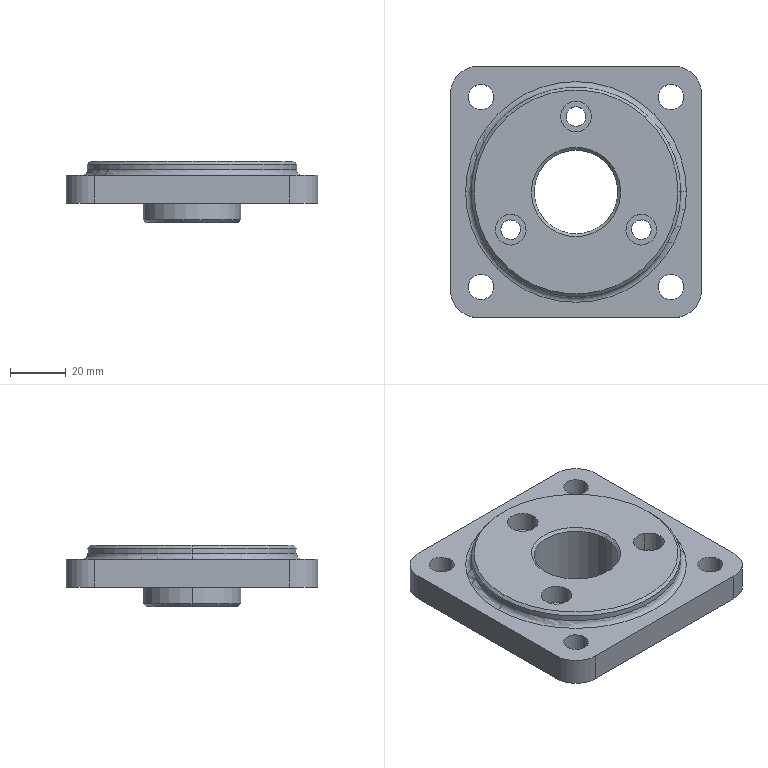Part | SolidWorks | features ICE 6, Fillet 2, Chamfer 1, CirPattern 1, Extrusion 1 | 1 solid | 49 faces | box 90 x 90 x 22 mm | volume 87928 mm3 | cylinder 30 | plane 11 | cone 6 | torus 2 | commonest cylinder face diameters 7 x6 9 x6 11 x6 20 x4 9.06 x2 30 x2
STEP:
#1=CARTESIAN_POINT('',(36.5,0.,15.));
#2=VERTEX_POINT('',#1);
#3=CARTESIAN_POINT('',(-36.5,0.,15.));
#4=VERTEX_POINT('',#3);
#5=CARTESIAN_POINT('',(0.,0.,15.));
#6=DIRECTION('',(0.,0.,1.));
#7=DIRECTION('',(1.,0.,0.));
#8=AXIS2_PLACEMENT_3D('',#5,#6,#7);
#9=CIRCLE('',#8,36.5);
#10=EDGE_CURVE('',#2,#4,#9,.T.);
#11=ORIENTED_EDGE('',*,*,#10,.F.);
#12=CARTESIAN_POINT('',(37.5,0.,14.));
#13=VERTEX_POINT('',#12);
#14=CARTESIAN_POINT('',(36.5,0.,15.));
#15=DIRECTION('',(0.7071,0.,-0.7071));
#16=VECTOR('',#15,1000.);
#17=LINE('',#14,#16);
#18=EDGE_CURVE('',#2,#13,#17,.T.);
#19=ORIENTED_EDGE('',*,*,#18,.T.);
#20=CARTESIAN_POINT('',(-37.5,0.,14.));
#21=VERTEX_POINT('',#20);
#22=CARTESIAN_POINT('',(0.,0.,14.));
#23=DIRECTION('',(0.,0.,-1.));
#24=DIRECTION('',(1.,0.,0.));
#25=AXIS2_PLACEMENT_3D('',#22,#23,#24);
#26=CIRCLE('',#25,37.5);
#27=EDGE_CURVE('',#21,#13,#26,.T.);
#28=ORIENTED_EDGE('',*,*,#27,.F.);
#29=CARTESIAN_POINT('',(-36.5,0.,15.));
#30=DIRECTION('',(-0.7071,0.,-0.7071));
#31=VECTOR('',#30,1000.);
#32=LINE('',#29,#31);
#33=EDGE_CURVE('',#4,#21,#32,.T.);
#34=ORIENTED_EDGE('',*,*,#33,.F.);
#35=EDGE_LOOP('',(#11,#19,#28,#34));
#36=FACE_OUTER_BOUND('',#35,.T.);
#37=CARTESIAN_POINT('',(0.,0.,15.));
#38=DIRECTION('',(0.,0.,-1.));
#39=DIRECTION('',(-1.,0.,0.));
#40=AXIS2_PLACEMENT_3D('',#37,#38,#39);
#41=CONICAL_SURFACE('',#40,36.5,0.7854);
#42=ADVANCED_FACE('',(#36),#41,.T.);
#43=CARTESIAN_POINT('',(-15.,0.,14.));
#44=VERTEX_POINT('',#43);
#45=CARTESIAN_POINT('',(15.,0.,14.));
#46=VERTEX_POINT('',#45);
#47=CARTESIAN_POINT('',(0.,0.,14.));
#48=DIRECTION('',(0.,0.,1.));
#49=DIRECTION('',(1.,0.,0.));
#50=AXIS2_PLACEMENT_3D('',#47,#48,#49);
#51=CIRCLE('',#50,15.);
#52=EDGE_CURVE('',#44,#46,#51,.T.);
#53=ORIENTED_EDGE('',*,*,#52,.F.);
#54=CARTESIAN_POINT('',(-16.,0.,15.));
#55=VERTEX_POINT('',#54);
#56=CARTESIAN_POINT('',(-15.,0.,14.));
#57=DIRECTION('',(-0.7071,0.,0.7071));
#58=VECTOR('',#57,1000.);
#59=LINE('',#56,#58);
#60=EDGE_CURVE('',#44,#55,#59,.T.);
#61=ORIENTED_EDGE('',*,*,#60,.T.);
#62=CARTESIAN_POINT('',(16.,0.,15.));
#63=VERTEX_POINT('',#62);
#64=CARTESIAN_POINT('',(0.,0.,15.));
#65=DIRECTION('',(0.,0.,-1.));
#66=DIRECTION('',(1.,0.,0.));
#67=AXIS2_PLACEMENT_3D('',#64,#65,#66);
#68=CIRCLE('',#67,16.);
#69=EDGE_CURVE('',#63,#55,#68,.T.);
#70=ORIENTED_EDGE('',*,*,#69,.F.);
#71=CARTESIAN_POINT('',(15.,0.,14.));
#72=DIRECTION('',(0.7071,0.,0.7071));
#73=VECTOR('',#72,1000.);
#74=LINE('',#71,#73);
#75=EDGE_CURVE('',#46,#63,#74,.T.);
#76=ORIENTED_EDGE('',*,*,#75,.F.);
#77=EDGE_LOOP('',(#53,#61,#70,#76));
#78=FACE_OUTER_BOUND('',#77,.T.);
#79=CARTESIAN_POINT('',(0.,0.,14.));
#80=DIRECTION('',(0.,0.,1.));
#81=DIRECTION('',(1.,0.,0.));
#82=AXIS2_PLACEMENT_3D('',#79,#80,#81);
#83=CONICAL_SURFACE('',#82,15.,0.7854);
#84=ADVANCED_FACE('',(#78),#83,.F.);
#85=CARTESIAN_POINT('',(-16.5,0.,-7.));
#86=VERTEX_POINT('',#85);
#87=CARTESIAN_POINT('',(16.5,0.,-7.));
#88=VERTEX_POINT('',#87);
#89=CARTESIAN_POINT('',(0.,0.,-7.));
#90=DIRECTION('',(0.,0.,-1.));
#91=DIRECTION('',(-1.,0.,0.));
#92=AXIS2_PLACEMENT_3D('',#89,#90,#91);
#93=CIRCLE('',#92,16.5);
#94=EDGE_CURVE('',#86,#88,#93,.T.);
#95=ORIENTED_EDGE('',*,*,#94,.F.);
#96=CARTESIAN_POINT('',(-17.5,0.,-6.));
#97=VERTEX_POINT('',#96);
#98=CARTESIAN_POINT('',(-16.5,0.,-7.));
#99=DIRECTION('',(-0.7071,0.,0.7071));
#100=VECTOR('',#99,1000.);
#101=LINE('',#98,#100);
#102=EDGE_CURVE('',#86,#97,#101,.T.);
#103=ORIENTED_EDGE('',*,*,#102,.T.);
#104=CARTESIAN_POINT('',(17.5,0.,-6.));
#105=VERTEX_POINT('',#104);
#106=CARTESIAN_POINT('',(0.,0.,-6.));
#107=DIRECTION('',(0.,0.,1.));
#108=DIRECTION('',(-1.,0.,0.));
#109=AXIS2_PLACEMENT_3D('',#106,#107,#108);
#110=CIRCLE('',#109,17.5);
#111=EDGE_CURVE('',#105,#97,#110,.T.);
#112=ORIENTED_EDGE('',*,*,#111,.F.);
#113=CARTESIAN_POINT('',(16.5,0.,-7.));
#114=DIRECTION('',(0.7071,0.,0.7071));
#115=VECTOR('',#114,1000.);
#116=LINE('',#113,#115);
#117=EDGE_CURVE('',#88,#105,#116,.T.);
#118=ORIENTED_EDGE('',*,*,#117,.F.);
#119=EDGE_LOOP('',(#95,#103,#112,#118));
#120=FACE_OUTER_BOUND('',#119,.T.);
#121=CARTESIAN_POINT('',(0.,0.,-7.));
#122=DIRECTION('',(0.,0.,1.));
#123=DIRECTION('',(1.,0.,0.));
#124=AXIS2_PLACEMENT_3D('',#121,#122,#123);
#125=CONICAL_SURFACE('',#124,16.5,0.7854);
#126=ADVANCED_FACE('',(#120),#125,.T.);
#127=CARTESIAN_POINT('',(-37.5,0.,12.));
#128=VERTEX_POINT('',#127);
#129=CARTESIAN_POINT('',(37.5,0.,12.));
#130=VERTEX_POINT('',#129);
#131=CARTESIAN_POINT('',(0.,0.,12.));
#132=DIRECTION('',(0.,0.,1.));
#133=DIRECTION('',(1.,0.,0.));
#134=AXIS2_PLACEMENT_3D('',#131,#132,#133);
#135=CIRCLE('',#134,37.5);
#136=EDGE_CURVE('',#128,#130,#135,.T.);
#137=ORIENTED_EDGE('',*,*,#136,.F.);
#138=CARTESIAN_POINT('',(-39.5,0.,10.));
#139=VERTEX_POINT('',#138);
#140=CARTESIAN_POINT('',(-39.5,0.,12.));
#141=DIRECTION('',(0.,1.,0.));
#142=DIRECTION('',(-1.,0.,0.));
#143=AXIS2_PLACEMENT_3D('',#140,#141,#142);
#144=CIRCLE('',#143,2.);
#145=EDGE_CURVE('',#128,#139,#144,.T.);
#146=ORIENTED_EDGE('',*,*,#145,.T.);
#147=CARTESIAN_POINT('',(39.5,0.,10.));
#148=VERTEX_POINT('',#147);
#149=CARTESIAN_POINT('',(0.,0.,10.));
#150=DIRECTION('',(0.,0.,-1.));
#151=DIRECTION('',(1.,0.,0.));
#152=AXIS2_PLACEMENT_3D('',#149,#150,#151);
#153=CIRCLE('',#152,39.5);
#154=EDGE_CURVE('',#148,#139,#153,.T.);
#155=ORIENTED_EDGE('',*,*,#154,.F.);
#156=CARTESIAN_POINT('',(39.5,0.,12.));
#157=DIRECTION('',(0.,-1.,0.));
#158=DIRECTION('',(0.,0.,-1.));
#159=AXIS2_PLACEMENT_3D('',#156,#157,#158);
#160=CIRCLE('',#159,2.);
#161=EDGE_CURVE('',#130,#148,#160,.T.);
#162=ORIENTED_EDGE('',*,*,#161,.F.);
#163=EDGE_LOOP('',(#137,#146,#155,#162));
#164=FACE_OUTER_BOUND('',#163,.T.);
#165=CARTESIAN_POINT('',(0.,0.,12.));
#166=DIRECTION('',(0.,0.,1.));
#167=DIRECTION('',(1.,0.,0.));
#168=AXIS2_PLACEMENT_3D('',#165,#166,#167);
#169=TOROIDAL_SURFACE('',#168,39.5,2.);
#170=ADVANCED_FACE('',(#164),#169,.F.);
#171=CARTESIAN_POINT('',(25.133,-10.469,0.));
#172=VERTEX_POINT('',#171);
#173=CARTESIAN_POINT('',(21.633,-16.531,0.));
#174=VERTEX_POINT('',#173);
#175=CARTESIAN_POINT('',(23.383,-13.5,0.));
#176=DIRECTION('',(0.,0.,1.));
#177=DIRECTION('',(-0.5,-0.866,0.));
#178=AXIS2_PLACEMENT_3D('',#175,#176,#177);
#179=CIRCLE('',#178,3.5);
#180=EDGE_CURVE('',#172,#174,#179,.T.);
#181=ORIENTED_EDGE('',*,*,#180,.F.);
#182=CARTESIAN_POINT('',(25.133,-10.469,8.));
#183=VERTEX_POINT('',#182);
#184=CARTESIAN_POINT('',(25.133,-10.469,-7.));
#185=DIRECTION('',(0.,0.,1.));
#186=VECTOR('',#185,1000.);
#187=LINE('',#184,#186);
#188=EDGE_CURVE('',#172,#183,#187,.T.);
#189=ORIENTED_EDGE('',*,*,#188,.T.);
#190=CARTESIAN_POINT('',(21.633,-16.531,8.));
#191=VERTEX_POINT('',#190);
#192=CARTESIAN_POINT('',(23.383,-13.5,8.));
#193=DIRECTION('',(0.,0.,1.));
#194=DIRECTION('',(-0.5,-0.866,0.));
#195=AXIS2_PLACEMENT_3D('',#192,#193,#194);
#196=CIRCLE('',#195,3.5);
#197=EDGE_CURVE('',#183,#191,#196,.T.);
#198=ORIENTED_EDGE('',*,*,#197,.T.);
#199=CARTESIAN_POINT('',(21.633,-16.531,-7.));
#200=DIRECTION('',(0.,0.,1.));
#201=VECTOR('',#200,1000.);
#202=LINE('',#199,#201);
#203=EDGE_CURVE('',#174,#191,#202,.T.);
#204=ORIENTED_EDGE('',*,*,#203,.F.);
#205=EDGE_LOOP('',(#181,#189,#198,#204));
#206=FACE_OUTER_BOUND('',#205,.T.);
#207=CARTESIAN_POINT('',(23.383,-13.5,-7.));
#208=DIRECTION('',(0.,0.,1.));
#209=DIRECTION('',(-0.5,-0.866,0.));
#210=AXIS2_PLACEMENT_3D('',#207,#208,#209);
#211=CYLINDRICAL_SURFACE('',#210,3.5);
#212=ADVANCED_FACE('',(#206),#211,.F.);
#213=CARTESIAN_POINT('',(26.133,-8.737,8.));
#214=VERTEX_POINT('',#213);
#215=CARTESIAN_POINT('',(20.633,-18.263,8.));
#216=VERTEX_POINT('',#215);
#217=CARTESIAN_POINT('',(23.383,-13.5,8.));
#218=DIRECTION('',(0.,0.,1.));
#219=DIRECTION('',(-0.5,-0.866,0.));
#220=AXIS2_PLACEMENT_3D('',#217,#218,#219);
#221=CIRCLE('',#220,5.5);
#222=EDGE_CURVE('',#214,#216,#221,.T.);
#223=ORIENTED_EDGE('',*,*,#222,.F.);
#224=CARTESIAN_POINT('',(26.133,-8.737,15.));
#225=VERTEX_POINT('',#224);
#226=CARTESIAN_POINT('',(26.133,-8.737,8.));
#227=DIRECTION('',(0.,0.,1.));
#228=VECTOR('',#227,1000.);
#229=LINE('',#226,#228);
#230=EDGE_CURVE('',#214,#225,#229,.T.);
#231=ORIENTED_EDGE('',*,*,#230,.T.);
#232=CARTESIAN_POINT('',(20.633,-18.263,15.));
#233=VERTEX_POINT('',#232);
#234=CARTESIAN_POINT('',(23.383,-13.5,15.));
#235=DIRECTION('',(0.,0.,1.));
#236=DIRECTION('',(-0.5,-0.866,0.));
#237=AXIS2_PLACEMENT_3D('',#234,#235,#236);
#238=CIRCLE('',#237,5.5);
#239=EDGE_CURVE('',#225,#233,#238,.T.);
#240=ORIENTED_EDGE('',*,*,#239,.T.);
#241=CARTESIAN_POINT('',(20.633,-18.263,8.));
#242=DIRECTION('',(0.,0.,1.));
#243=VECTOR('',#242,1000.);
#244=LINE('',#241,#243);
#245=EDGE_CURVE('',#216,#233,#244,.T.);
#246=ORIENTED_EDGE('',*,*,#245,.F.);
#247=EDGE_LOOP('',(#223,#231,#240,#246));
#248=FACE_OUTER_BOUND('',#247,.T.);
#249=CARTESIAN_POINT('',(23.383,-13.5,8.));
#250=DIRECTION('',(0.,0.,1.));
#251=DIRECTION('',(-0.5,-0.866,0.));
#252=AXIS2_PLACEMENT_3D('',#249,#250,#251);
#253=CYLINDRICAL_SURFACE('',#252,5.5);
#254=ADVANCED_FACE('',(#248),#253,.F.);
#255=CARTESIAN_POINT('',(-21.633,-16.531,0.));
#256=VERTEX_POINT('',#255);
#257=CARTESIAN_POINT('',(-25.133,-10.469,0.));
#258=VERTEX_POINT('',#257);
#259=CARTESIAN_POINT('',(-23.383,-13.5,0.));
#260=DIRECTION('',(0.,0.,1.));
#261=DIRECTION('',(-0.5,0.866,0.));
#262=AXIS2_PLACEMENT_3D('',#259,#260,#261);
#263=CIRCLE('',#262,3.5);
#264=EDGE_CURVE('',#256,#258,#263,.T.);
#265=ORIENTED_EDGE('',*,*,#264,.F.);
#266=CARTESIAN_POINT('',(-21.633,-16.531,8.));
#267=VERTEX_POINT('',#266);
#268=CARTESIAN_POINT('',(-21.633,-16.531,-7.));
#269=DIRECTION('',(0.,0.,1.));
#270=VECTOR('',#269,1000.);
#271=LINE('',#268,#270);
#272=EDGE_CURVE('',#256,#267,#271,.T.);
#273=ORIENTED_EDGE('',*,*,#272,.T.);
#274=CARTESIAN_POINT('',(-25.133,-10.469,8.));
#275=VERTEX_POINT('',#274);
#276=CARTESIAN_POINT('',(-23.383,-13.5,8.));
#277=DIRECTION('',(0.,0.,1.));
#278=DIRECTION('',(-0.5,0.866,0.));
#279=AXIS2_PLACEMENT_3D('',#276,#277,#278);
#280=CIRCLE('',#279,3.5);
#281=EDGE_CURVE('',#267,#275,#280,.T.);
#282=ORIENTED_EDGE('',*,*,#281,.T.);
#283=CARTESIAN_POINT('',(-25.133,-10.469,-7.));
#284=DIRECTION('',(0.,0.,1.));
#285=VECTOR('',#284,1000.);
#286=LINE('',#283,#285);
#287=EDGE_CURVE('',#258,#275,#286,.T.);
#288=ORIENTED_EDGE('',*,*,#287,.F.);
#289=EDGE_LOOP('',(#265,#273,#282,#288));
#290=FACE_OUTER_BOUND('',#289,.T.);
#291=CARTESIAN_POINT('',(-23.383,-13.5,-7.));
#292=DIRECTION('',(0.,0.,1.));
#293=DIRECTION('',(-0.5,0.866,0.));
#294=AXIS2_PLACEMENT_3D('',#291,#292,#293);
#295=CYLINDRICAL_SURFACE('',#294,3.5);
#296=ADVANCED_FACE('',(#290),#295,.F.);
#297=CARTESIAN_POINT('',(-20.633,-18.263,8.));
#298=VERTEX_POINT('',#297);
#299=CARTESIAN_POINT('',(-26.133,-8.737,8.));
#300=VERTEX_POINT('',#299);
#301=CARTESIAN_POINT('',(-23.383,-13.5,8.));
#302=DIRECTION('',(0.,0.,1.));
#303=DIRECTION('',(-0.5,0.866,0.));
#304=AXIS2_PLACEMENT_3D('',#301,#302,#303);
#305=CIRCLE('',#304,5.5);
#306=EDGE_CURVE('',#298,#300,#305,.T.);
#307=ORIENTED_EDGE('',*,*,#306,.F.);
#308=CARTESIAN_POINT('',(-20.633,-18.263,15.));
#309=VERTEX_POINT('',#308);
#310=CARTESIAN_POINT('',(-20.633,-18.263,8.));
#311=DIRECTION('',(0.,0.,1.));
#312=VECTOR('',#311,1000.);
#313=LINE('',#310,#312);
#314=EDGE_CURVE('',#298,#309,#313,.T.);
#315=ORIENTED_EDGE('',*,*,#314,.T.);
#316=CARTESIAN_POINT('',(-26.133,-8.737,15.));
#317=VERTEX_POINT('',#316);
#318=CARTESIAN_POINT('',(-23.383,-13.5,15.));
#319=DIRECTION('',(0.,0.,1.));
#320=DIRECTION('',(-0.5,0.866,0.));
#321=AXIS2_PLACEMENT_3D('',#318,#319,#320);
#322=CIRCLE('',#321,5.5);
#323=EDGE_CURVE('',#309,#317,#322,.T.);
#324=ORIENTED_EDGE('',*,*,#323,.T.);
#325=CARTESIAN_POINT('',(-26.133,-8.737,8.));
#326=DIRECTION('',(0.,0.,1.));
#327=VECTOR('',#326,1000.);
#328=LINE('',#325,#327);
#329=EDGE_CURVE('',#300,#317,#328,.T.);
#330=ORIENTED_EDGE('',*,*,#329,.F.);
#331=EDGE_LOOP('',(#307,#315,#324,#330));
#332=FACE_OUTER_BOUND('',#331,.T.);
#333=CARTESIAN_POINT('',(-23.383,-13.5,8.));
#334=DIRECTION('',(0.,0.,1.));
#335=DIRECTION('',(-0.5,0.866,0.));
#336=AXIS2_PLACEMENT_3D('',#333,#334,#335);
#337=CYLINDRICAL_SURFACE('',#336,5.5);
#338=ADVANCED_FACE('',(#332),#337,.F.);
#339=CARTESIAN_POINT('',(-3.5,27.,0.));
#340=VERTEX_POINT('',#339);
#341=CARTESIAN_POINT('',(3.5,27.,0.));
#342=VERTEX_POINT('',#341);
#343=CARTESIAN_POINT('',(0.,27.,0.));
#344=DIRECTION('',(0.,0.,1.));
#345=DIRECTION('',(1.,0.,0.));
#346=AXIS2_PLACEMENT_3D('',#343,#344,#345);
#347=CIRCLE('',#346,3.5);
#348=EDGE_CURVE('',#340,#342,#347,.T.);
#349=ORIENTED_EDGE('',*,*,#348,.F.);
#350=CARTESIAN_POINT('',(-3.5,27.,8.));
#351=VERTEX_POINT('',#350);
#352=CARTESIAN_POINT('',(-3.5,27.,-7.));
#353=DIRECTION('',(0.,0.,1.));
#354=VECTOR('',#353,1000.);
#355=LINE('',#352,#354);
#356=EDGE_CURVE('',#340,#351,#355,.T.);
#357=ORIENTED_EDGE('',*,*,#356,.T.);
#358=CARTESIAN_POINT('',(3.5,27.,8.));
#359=VERTEX_POINT('',#358);
#360=CARTESIAN_POINT('',(0.,27.,8.));
#361=DIRECTION('',(0.,0.,1.));
#362=DIRECTION('',(1.,0.,0.));
#363=AXIS2_PLACEMENT_3D('',#360,#361,#362);
#364=CIRCLE('',#363,3.5);
#365=EDGE_CURVE('',#351,#359,#364,.T.);
#366=ORIENTED_EDGE('',*,*,#365,.T.);
#367=CARTESIAN_POINT('',(3.5,27.,-7.));
#368=DIRECTION('',(0.,0.,1.));
#369=VECTOR('',#368,1000.);
#370=LINE('',#367,#369);
#371=EDGE_CURVE('',#342,#359,#370,.T.);
#372=ORIENTED_EDGE('',*,*,#371,.F.);
#373=EDGE_LOOP('',(#349,#357,#366,#372));
#374=FACE_OUTER_BOUND('',#373,.T.);
#375=CARTESIAN_POINT('',(0.,27.,-7.));
#376=DIRECTION('',(0.,0.,1.));
#377=DIRECTION('',(1.,0.,0.));
#378=AXIS2_PLACEMENT_3D('',#375,#376,#377);
#379=CYLINDRICAL_SURFACE('',#378,3.5);
#380=ADVANCED_FACE('',(#374),#379,.F.);
#381=CARTESIAN_POINT('',(-5.5,27.,8.));
#382=VERTEX_POINT('',#381);
#383=CARTESIAN_POINT('',(5.5,27.,8.));
#384=VERTEX_POINT('',#383);
#385=CARTESIAN_POINT('',(0.,27.,8.));
#386=DIRECTION('',(0.,0.,1.));
#387=DIRECTION('',(1.,0.,0.));
#388=AXIS2_PLACEMENT_3D('',#385,#386,#387);
#389=CIRCLE('',#388,5.5);
#390=EDGE_CURVE('',#382,#384,#389,.T.);
#391=ORIENTED_EDGE('',*,*,#390,.F.);
#392=CARTESIAN_POINT('',(-5.5,27.,15.));
#393=VERTEX_POINT('',#392);
#394=CARTESIAN_POINT('',(-5.5,27.,8.));
#395=DIRECTION('',(0.,0.,1.));
#396=VECTOR('',#395,1000.);
#397=LINE('',#394,#396);
#398=EDGE_CURVE('',#382,#393,#397,.T.);
#399=ORIENTED_EDGE('',*,*,#398,.T.);
#400=CARTESIAN_POINT('',(5.5,27.,15.));
#401=VERTEX_POINT('',#400);
#402=CARTESIAN_POINT('',(0.,27.,15.));
#403=DIRECTION('',(0.,0.,1.));
#404=DIRECTION('',(1.,0.,0.));
#405=AXIS2_PLACEMENT_3D('',#402,#403,#404);
#406=CIRCLE('',#405,5.5);
#407=EDGE_CURVE('',#393,#401,#406,.T.);
#408=ORIENTED_EDGE('',*,*,#407,.T.);
#409=CARTESIAN_POINT('',(5.5,27.,8.));
#410=DIRECTION('',(0.,0.,1.));
#411=VECTOR('',#410,1000.);
#412=LINE('',#409,#411);
#413=EDGE_CURVE('',#384,#401,#412,.T.);
#414=ORIENTED_EDGE('',*,*,#413,.F.);
#415=EDGE_LOOP('',(#391,#399,#408,#414));
#416=FACE_OUTER_BOUND('',#415,.T.);
#417=CARTESIAN_POINT('',(0.,27.,8.));
#418=DIRECTION('',(0.,0.,1.));
#419=DIRECTION('',(1.,0.,0.));
#420=AXIS2_PLACEMENT_3D('',#417,#418,#419);
#421=CYLINDRICAL_SURFACE('',#420,5.5);
#422=ADVANCED_FACE('',(#416),#421,.F.);
#423=CARTESIAN_POINT('',(-15.,0.,-7.));
#424=VERTEX_POINT('',#423);
#425=CARTESIAN_POINT('',(15.,0.,-7.));
#426=VERTEX_POINT('',#425);
#427=CARTESIAN_POINT('',(0.,0.,-7.));
#428=DIRECTION('',(0.,0.,1.));
#429=DIRECTION('',(1.,0.,0.));
#430=AXIS2_PLACEMENT_3D('',#427,#428,#429);
#431=CIRCLE('',#430,15.);
#432=EDGE_CURVE('',#424,#426,#431,.T.);
#433=ORIENTED_EDGE('',*,*,#432,.F.);
#434=CARTESIAN_POINT('',(-15.,0.,-7.));
#435=DIRECTION('',(0.,0.,1.));
#436=VECTOR('',#435,1000.);
#437=LINE('',#434,#436);
#438=EDGE_CURVE('',#424,#44,#437,.T.);
#439=ORIENTED_EDGE('',*,*,#438,.T.);
#440=ORIENTED_EDGE('',*,*,#52,.T.);
#441=CARTESIAN_POINT('',(15.,0.,-7.));
#442=DIRECTION('',(0.,0.,1.));
#443=VECTOR('',#442,1000.);
#444=LINE('',#441,#443);
#445=EDGE_CURVE('',#426,#46,#444,.T.);
#446=ORIENTED_EDGE('',*,*,#445,.F.);
#447=EDGE_LOOP('',(#433,#439,#440,#446));
#448=FACE_OUTER_BOUND('',#447,.T.);
#449=CARTESIAN_POINT('',(0.,0.,-7.));
#450=DIRECTION('',(0.,0.,1.));
#451=DIRECTION('',(1.,0.,0.));
#452=AXIS2_PLACEMENT_3D('',#449,#450,#451);
#453=CYLINDRICAL_SURFACE('',#452,15.);
#454=ADVANCED_FACE('',(#448),#453,.F.);
#455=ORIENTED_EDGE('',*,*,#111,.T.);
#456=CARTESIAN_POINT('',(-17.5,0.,0.));
#457=VERTEX_POINT('',#456);
#458=CARTESIAN_POINT('',(-17.5,0.,-7.));
#459=DIRECTION('',(0.,0.,1.));
#460=VECTOR('',#459,1000.);
#461=LINE('',#458,#460);
#462=EDGE_CURVE('',#97,#457,#461,.T.);
#463=ORIENTED_EDGE('',*,*,#462,.T.);
#464=CARTESIAN_POINT('',(17.5,0.,0.));
#465=VERTEX_POINT('',#464);
#466=CARTESIAN_POINT('',(0.,0.,0.));
#467=DIRECTION('',(0.,0.,-1.));
#468=DIRECTION('',(1.,0.,0.));
#469=AXIS2_PLACEMENT_3D('',#466,#467,#468);
#470=CIRCLE('',#469,17.5);
#471=EDGE_CURVE('',#457,#465,#470,.T.);
#472=ORIENTED_EDGE('',*,*,#471,.T.);
#473=CARTESIAN_POINT('',(17.5,0.,-7.));
#474=DIRECTION('',(0.,0.,1.));
#475=VECTOR('',#474,1000.);
#476=LINE('',#473,#475);
#477=EDGE_CURVE('',#105,#465,#476,.T.);
#478=ORIENTED_EDGE('',*,*,#477,.F.);
#479=EDGE_LOOP('',(#455,#463,#472,#478));
#480=FACE_OUTER_BOUND('',#479,.T.);
#481=CARTESIAN_POINT('',(0.,0.,-7.));
#482=DIRECTION('',(0.,0.,1.));
#483=DIRECTION('',(1.,0.,0.));
#484=AXIS2_PLACEMENT_3D('',#481,#482,#483);
#485=CYLINDRICAL_SURFACE('',#484,17.5);
#486=ADVANCED_FACE('',(#480),#485,.T.);
#487=ORIENTED_EDGE('',*,*,#27,.T.);
#488=CARTESIAN_POINT('',(37.5,0.,15.));
#489=DIRECTION('',(0.,0.,-1.));
#490=VECTOR('',#489,1000.);
#491=LINE('',#488,#490);
#492=EDGE_CURVE('',#13,#130,#491,.T.);
#493=ORIENTED_EDGE('',*,*,#492,.T.);
#494=CARTESIAN_POINT('',(0.,0.,12.));
#495=DIRECTION('',(0.,0.,1.));
#496=DIRECTION('',(1.,0.,0.));
#497=AXIS2_PLACEMENT_3D('',#494,#495,#496);
#498=CIRCLE('',#497,37.5);
#499=EDGE_CURVE('',#130,#128,#498,.T.);
#500=ORIENTED_EDGE('',*,*,#499,.T.);
#501=CARTESIAN_POINT('',(-37.5,0.,15.));
#502=DIRECTION('',(0.,0.,-1.));
#503=VECTOR('',#502,1000.);
#504=LINE('',#501,#503);
#505=EDGE_CURVE('',#21,#128,#504,.T.);
#506=ORIENTED_EDGE('',*,*,#505,.F.);
#507=EDGE_LOOP('',(#487,#493,#500,#506));
#508=FACE_OUTER_BOUND('',#507,.T.);
#509=CARTESIAN_POINT('',(0.,0.,15.));
#510=DIRECTION('',(0.,0.,-1.));
#511=DIRECTION('',(-1.,0.,0.));
#512=AXIS2_PLACEMENT_3D('',#509,#510,#511);
#513=CYLINDRICAL_SURFACE('',#512,37.5);
#514=ADVANCED_FACE('',(#508),#513,.T.);
#515=CARTESIAN_POINT('',(29.5,34.,0.));
#516=VERTEX_POINT('',#515);
#517=CARTESIAN_POINT('',(38.5,34.,0.));
#518=VERTEX_POINT('',#517);
#519=CARTESIAN_POINT('',(34.,34.,0.));
#520=DIRECTION('',(0.,0.,1.));
#521=DIRECTION('',(1.,0.,0.));
#522=AXIS2_PLACEMENT_3D('',#519,#520,#521);
#523=CIRCLE('',#522,4.5);
#524=EDGE_CURVE('',#516,#518,#523,.T.);
#525=ORIENTED_EDGE('',*,*,#524,.F.);
#526=CARTESIAN_POINT('',(29.5,34.,10.));
#527=VERTEX_POINT('',#526);
#528=CARTESIAN_POINT('',(29.5,34.,0.));
#529=DIRECTION('',(0.,0.,1.));
#530=VECTOR('',#529,1000.);
#531=LINE('',#528,#530);
#532=EDGE_CURVE('',#516,#527,#531,.T.);
#533=ORIENTED_EDGE('',*,*,#532,.T.);
#534=CARTESIAN_POINT('',(38.5,34.,10.));
#535=VERTEX_POINT('',#534);
#536=CARTESIAN_POINT('',(34.,34.,10.));
#537=DIRECTION('',(0.,0.,1.));
#538=DIRECTION('',(1.,0.,0.));
#539=AXIS2_PLACEMENT_3D('',#536,#537,#538);
#540=CIRCLE('',#539,4.5);
#541=EDGE_CURVE('',#527,#535,#540,.T.);
#542=ORIENTED_EDGE('',*,*,#541,.T.);
#543=CARTESIAN_POINT('',(38.5,34.,0.));
#544=DIRECTION('',(0.,0.,1.));
#545=VECTOR('',#544,1000.);
#546=LINE('',#543,#545);
#547=EDGE_CURVE('',#518,#535,#546,.T.);
#548=ORIENTED_EDGE('',*,*,#547,.F.);
#549=EDGE_LOOP('',(#525,#533,#542,#548));
#550=FACE_OUTER_BOUND('',#549,.T.);
#551=CARTESIAN_POINT('',(34.,34.,0.));
#552=DIRECTION('',(0.,0.,1.));
#553=DIRECTION('',(1.,0.,0.));
#554=AXIS2_PLACEMENT_3D('',#551,#552,#553);
#555=CYLINDRICAL_SURFACE('',#554,4.5);
#556=ADVANCED_FACE('',(#550),#555,.F.);
#557=CARTESIAN_POINT('',(-38.5,-34.,0.));
#558=VERTEX_POINT('',#557);
#559=CARTESIAN_POINT('',(-29.5,-34.,0.));
#560=VERTEX_POINT('',#559);
#561=CARTESIAN_POINT('',(-34.,-34.,0.));
#562=DIRECTION('',(0.,0.,1.));
#563=DIRECTION('',(1.,0.,0.));
#564=AXIS2_PLACEMENT_3D('',#561,#562,#563);
#565=CIRCLE('',#564,4.5);
#566=EDGE_CURVE('',#558,#560,#565,.T.);
#567=ORIENTED_EDGE('',*,*,#566,.F.);
#568=CARTESIAN_POINT('',(-38.5,-34.,10.));
#569=VERTEX_POINT('',#568);
#570=CARTESIAN_POINT('',(-38.5,-34.,0.));
#571=DIRECTION('',(0.,0.,1.));
#572=VECTOR('',#571,1000.);
#573=LINE('',#570,#572);
#574=EDGE_CURVE('',#558,#569,#573,.T.);
#575=ORIENTED_EDGE('',*,*,#574,.T.);
#576=CARTESIAN_POINT('',(-29.5,-34.,10.));
#577=VERTEX_POINT('',#576);
#578=CARTESIAN_POINT('',(-34.,-34.,10.));
#579=DIRECTION('',(0.,0.,1.));
#580=DIRECTION('',(1.,0.,0.));
#581=AXIS2_PLACEMENT_3D('',#578,#579,#580);
#582=CIRCLE('',#581,4.5);
#583=EDGE_CURVE('',#569,#577,#582,.T.);
#584=ORIENTED_EDGE('',*,*,#583,.T.);
#585=CARTESIAN_POINT('',(-29.5,-34.,0.));
#586=DIRECTION('',(0.,0.,1.));
#587=VECTOR('',#586,1000.);
#588=LINE('',#585,#587);
#589=EDGE_CURVE('',#560,#577,#588,.T.);
#590=ORIENTED_EDGE('',*,*,#589,.F.);
#591=EDGE_LOOP('',(#567,#575,#584,#590));
#592=FACE_OUTER_BOUND('',#591,.T.);
#593=CARTESIAN_POINT('',(-34.,-34.,0.));
#594=DIRECTION('',(0.,0.,1.));
#595=DIRECTION('',(1.,0.,0.));
#596=AXIS2_PLACEMENT_3D('',#593,#594,#595);
#597=CYLINDRICAL_SURFACE('',#596,4.5);
#598=ADVANCED_FACE('',(#592),#597,.F.);
#599=CARTESIAN_POINT('',(29.47,-34.,0.));
#600=VERTEX_POINT('',#599);
#601=CARTESIAN_POINT('',(38.53,-34.,0.));
#602=VERTEX_POINT('',#601);
#603=CARTESIAN_POINT('',(34.,-34.,0.));
#604=DIRECTION('',(0.,0.,1.));
#605=DIRECTION('',(1.,0.,0.));
#606=AXIS2_PLACEMENT_3D('',#603,#604,#605);
#607=CIRCLE('',#606,4.53);
#608=EDGE_CURVE('',#600,#602,#607,.T.);
#609=ORIENTED_EDGE('',*,*,#608,.F.);
#610=CARTESIAN_POINT('',(29.47,-34.,10.));
#611=VERTEX_POINT('',#610);
#612=CARTESIAN_POINT('',(29.47,-34.,0.));
#613=DIRECTION('',(0.,0.,1.));
#614=VECTOR('',#613,1000.);
#615=LINE('',#612,#614);
#616=EDGE_CURVE('',#600,#611,#615,.T.);
#617=ORIENTED_EDGE('',*,*,#616,.T.);
#618=CARTESIAN_POINT('',(38.53,-34.,10.));
#619=VERTEX_POINT('',#618);
#620=CARTESIAN_POINT('',(34.,-34.,10.));
#621=DIRECTION('',(0.,0.,1.));
#622=DIRECTION('',(1.,0.,0.));
#623=AXIS2_PLACEMENT_3D('',#620,#621,#622);
#624=CIRCLE('',#623,4.53);
#625=EDGE_CURVE('',#611,#619,#624,.T.);
#626=ORIENTED_EDGE('',*,*,#625,.T.);
#627=CARTESIAN_POINT('',(38.53,-34.,0.));
#628=DIRECTION('',(0.,0.,1.));
#629=VECTOR('',#628,1000.);
#630=LINE('',#627,#629);
#631=EDGE_CURVE('',#602,#619,#630,.T.);
#632=ORIENTED_EDGE('',*,*,#631,.F.);
#633=EDGE_LOOP('',(#609,#617,#626,#632));
#634=FACE_OUTER_BOUND('',#633,.T.);
#635=CARTESIAN_POINT('',(34.,-34.,0.));
#636=DIRECTION('',(0.,0.,1.));
#637=DIRECTION('',(1.,0.,0.));
#638=AXIS2_PLACEMENT_3D('',#635,#636,#637);
#639=CYLINDRICAL_SURFACE('',#638,4.53);
#640=ADVANCED_FACE('',(#634),#639,.F.);
#641=CARTESIAN_POINT('',(-38.5,34.,0.));
#642=VERTEX_POINT('',#641);
#643=CARTESIAN_POINT('',(-29.5,34.,0.));
#644=VERTEX_POINT('',#643);
#645=CARTESIAN_POINT('',(-34.,34.,0.));
#646=DIRECTION('',(0.,0.,1.));
#647=DIRECTION('',(1.,0.,0.));
#648=AXIS2_PLACEMENT_3D('',#645,#646,#647);
#649=CIRCLE('',#648,4.5);
#650=EDGE_CURVE('',#642,#644,#649,.T.);
#651=ORIENTED_EDGE('',*,*,#650,.F.);
#652=CARTESIAN_POINT('',(-38.5,34.,10.));
#653=VERTEX_POINT('',#652);
#654=CARTESIAN_POINT('',(-38.5,34.,0.));
#655=DIRECTION('',(0.,0.,1.));
#656=VECTOR('',#655,1000.);
#657=LINE('',#654,#656);
#658=EDGE_CURVE('',#642,#653,#657,.T.);
#659=ORIENTED_EDGE('',*,*,#658,.T.);
#660=CARTESIAN_POINT('',(-29.5,34.,10.));
#661=VERTEX_POINT('',#660);
#662=CARTESIAN_POINT('',(-34.,34.,10.));
#663=DIRECTION('',(0.,0.,1.));
#664=DIRECTION('',(1.,0.,0.));
#665=AXIS2_PLACEMENT_3D('',#662,#663,#664);
#666=CIRCLE('',#665,4.5);
#667=EDGE_CURVE('',#653,#661,#666,.T.);
#668=ORIENTED_EDGE('',*,*,#667,.T.);
#669=CARTESIAN_POINT('',(-29.5,34.,0.));
#670=DIRECTION('',(0.,0.,1.));
#671=VECTOR('',#670,1000.);
#672=LINE('',#669,#671);
#673=EDGE_CURVE('',#644,#661,#672,.T.);
#674=ORIENTED_EDGE('',*,*,#673,.F.);
#675=EDGE_LOOP('',(#651,#659,#668,#674));
#676=FACE_OUTER_BOUND('',#675,.T.);
#677=CARTESIAN_POINT('',(-34.,34.,0.));
#678=DIRECTION('',(0.,0.,1.));
#679=DIRECTION('',(1.,0.,0.));
#680=AXIS2_PLACEMENT_3D('',#677,#678,#679);
#681=CYLINDRICAL_SURFACE('',#680,4.5);
#682=ADVANCED_FACE('',(#676),#681,.F.);
#683=CARTESIAN_POINT('',(45.,-35.,10.));
#684=VERTEX_POINT('',#683);
#685=CARTESIAN_POINT('',(45.,35.,10.));
#686=VERTEX_POINT('',#685);
#687=CARTESIAN_POINT('',(45.,45.,10.));
#688=DIRECTION('',(0.,1.,0.));
#689=VECTOR('',#688,1000.);
#690=LINE('',#687,#689);
#691=EDGE_CURVE('',#684,#686,#690,.T.);
#692=ORIENTED_EDGE('',*,*,#691,.F.);
#693=CARTESIAN_POINT('',(45.,-35.,0.));
#694=VERTEX_POINT('',#693);
#695=CARTESIAN_POINT('',(45.,-35.,10.));
#696=DIRECTION('',(0.,0.,-1.));
#697=VECTOR('',#696,1000.);
#698=LINE('',#695,#697);
#699=EDGE_CURVE('',#684,#694,#698,.T.);
#700=ORIENTED_EDGE('',*,*,#699,.T.);
#701=CARTESIAN_POINT('',(45.,35.,0.));
#702=VERTEX_POINT('',#701);
#703=CARTESIAN_POINT('',(45.,45.,0.));
#704=DIRECTION('',(0.,1.,0.));
#705=VECTOR('',#704,1000.);
#706=LINE('',#703,#705);
#707=EDGE_CURVE('',#694,#702,#706,.T.);
#708=ORIENTED_EDGE('',*,*,#707,.T.);
#709=CARTESIAN_POINT('',(45.,35.,10.));
#710=DIRECTION('',(0.,0.,1.));
#711=VECTOR('',#710,1000.);
#712=LINE('',#709,#711);
#713=EDGE_CURVE('',#702,#686,#712,.T.);
#714=ORIENTED_EDGE('',*,*,#713,.T.);
#715=EDGE_LOOP('',(#692,#700,#708,#714));
#716=FACE_OUTER_BOUND('',#715,.T.);
#717=CARTESIAN_POINT('',(45.,45.,10.));
#718=DIRECTION('',(-1.,0.,0.));
#719=DIRECTION('',(0.,-1.,0.));
#720=AXIS2_PLACEMENT_3D('',#717,#718,#719);
#721=PLANE('',#720);
#722=ADVANCED_FACE('',(#716),#721,.F.);
#723=CARTESIAN_POINT('',(35.,45.,10.));
#724=VERTEX_POINT('',#723);
#725=CARTESIAN_POINT('',(-35.,45.,10.));
#726=VERTEX_POINT('',#725);
#727=CARTESIAN_POINT('',(-45.,45.,10.));
#728=DIRECTION('',(-1.,0.,0.));
#729=VECTOR('',#728,1000.);
#730=LINE('',#727,#729);
#731=EDGE_CURVE('',#724,#726,#730,.T.);
#732=ORIENTED_EDGE('',*,*,#731,.F.);
#733=CARTESIAN_POINT('',(35.,45.,0.));
#734=VERTEX_POINT('',#733);
#735=CARTESIAN_POINT('',(35.,45.,10.));
#736=DIRECTION('',(0.,0.,-1.));
#737=VECTOR('',#736,1000.);
#738=LINE('',#735,#737);
#739=EDGE_CURVE('',#724,#734,#738,.T.);
#740=ORIENTED_EDGE('',*,*,#739,.T.);
#741=CARTESIAN_POINT('',(-35.,45.,0.));
#742=VERTEX_POINT('',#741);
#743=CARTESIAN_POINT('',(-45.,45.,0.));
#744=DIRECTION('',(-1.,0.,0.));
#745=VECTOR('',#744,1000.);
#746=LINE('',#743,#745);
#747=EDGE_CURVE('',#734,#742,#746,.T.);
#748=ORIENTED_EDGE('',*,*,#747,.T.);
#749=CARTESIAN_POINT('',(-35.,45.,10.));
#750=DIRECTION('',(0.,0.,1.));
#751=VECTOR('',#750,1000.);
#752=LINE('',#749,#751);
#753=EDGE_CURVE('',#742,#726,#752,.T.);
#754=ORIENTED_EDGE('',*,*,#753,.T.);
#755=EDGE_LOOP('',(#732,#740,#748,#754));
#756=FACE_OUTER_BOUND('',#755,.T.);
#757=CARTESIAN_POINT('',(-45.,45.,10.));
#758=DIRECTION('',(0.,-1.,0.));
#759=DIRECTION('',(0.,0.,-1.));
#760=AXIS2_PLACEMENT_3D('',#757,#758,#759);
#761=PLANE('',#760);
#762=ADVANCED_FACE('',(#756),#761,.F.);
#763=CARTESIAN_POINT('',(-45.,35.,0.));
#764=VERTEX_POINT('',#763);
#765=CARTESIAN_POINT('',(-45.,-35.,0.));
#766=VERTEX_POINT('',#765);
#767=CARTESIAN_POINT('',(-45.,45.,0.));
#768=DIRECTION('',(0.,-1.,0.));
#769=VECTOR('',#768,1000.);
#770=LINE('',#767,#769);
#771=EDGE_CURVE('',#764,#766,#770,.T.);
#772=ORIENTED_EDGE('',*,*,#771,.T.);
#773=CARTESIAN_POINT('',(-45.,-35.,10.));
#774=VERTEX_POINT('',#773);
#775=CARTESIAN_POINT('',(-45.,-35.,10.));
#776=DIRECTION('',(0.,0.,1.));
#777=VECTOR('',#776,1000.);
#778=LINE('',#775,#777);
#779=EDGE_CURVE('',#766,#774,#778,.T.);
#780=ORIENTED_EDGE('',*,*,#779,.T.);
#781=CARTESIAN_POINT('',(-45.,35.,10.));
#782=VERTEX_POINT('',#781);
#783=CARTESIAN_POINT('',(-45.,45.,10.));
#784=DIRECTION('',(0.,-1.,0.));
#785=VECTOR('',#784,1000.);
#786=LINE('',#783,#785);
#787=EDGE_CURVE('',#782,#774,#786,.T.);
#788=ORIENTED_EDGE('',*,*,#787,.F.);
#789=CARTESIAN_POINT('',(-45.,35.,10.));
#790=DIRECTION('',(0.,0.,-1.));
#791=VECTOR('',#790,1000.);
#792=LINE('',#789,#791);
#793=EDGE_CURVE('',#782,#764,#792,.T.);
#794=ORIENTED_EDGE('',*,*,#793,.T.);
#795=EDGE_LOOP('',(#772,#780,#788,#794));
#796=FACE_OUTER_BOUND('',#795,.T.);
#797=CARTESIAN_POINT('',(-45.,45.,10.));
#798=DIRECTION('',(1.,0.,0.));
#799=DIRECTION('',(0.,1.,0.));
#800=AXIS2_PLACEMENT_3D('',#797,#798,#799);
#801=PLANE('',#800);
#802=ADVANCED_FACE('',(#796),#801,.F.);
#803=CARTESIAN_POINT('',(-35.,-45.,10.));
#804=VERTEX_POINT('',#803);
#805=CARTESIAN_POINT('',(35.,-45.,10.));
#806=VERTEX_POINT('',#805);
#807=CARTESIAN_POINT('',(-45.,-45.,10.));
#808=DIRECTION('',(1.,0.,0.));
#809=VECTOR('',#808,1000.);
#810=LINE('',#807,#809);
#811=EDGE_CURVE('',#804,#806,#810,.T.);
#812=ORIENTED_EDGE('',*,*,#811,.F.);
#813=CARTESIAN_POINT('',(-35.,-45.,0.));
#814=VERTEX_POINT('',#813);
#815=CARTESIAN_POINT('',(-35.,-45.,10.));
#816=DIRECTION('',(0.,0.,-1.));
#817=VECTOR('',#816,1000.);
#818=LINE('',#815,#817);
#819=EDGE_CURVE('',#804,#814,#818,.T.);
#820=ORIENTED_EDGE('',*,*,#819,.T.);
#821=CARTESIAN_POINT('',(35.,-45.,0.));
#822=VERTEX_POINT('',#821);
#823=CARTESIAN_POINT('',(-45.,-45.,0.));
#824=DIRECTION('',(1.,0.,0.));
#825=VECTOR('',#824,1000.);
#826=LINE('',#823,#825);
#827=EDGE_CURVE('',#814,#822,#826,.T.);
#828=ORIENTED_EDGE('',*,*,#827,.T.);
#829=CARTESIAN_POINT('',(35.,-45.,10.));
#830=DIRECTION('',(0.,0.,1.));
#831=VECTOR('',#830,1000.);
#832=LINE('',#829,#831);
#833=EDGE_CURVE('',#822,#806,#832,.T.);
#834=ORIENTED_EDGE('',*,*,#833,.T.);
#835=EDGE_LOOP('',(#812,#820,#828,#834));
#836=FACE_OUTER_BOUND('',#835,.T.);
#837=CARTESIAN_POINT('',(-45.,-45.,10.));
#838=DIRECTION('',(0.,1.,0.));
#839=DIRECTION('',(0.,0.,1.));
#840=AXIS2_PLACEMENT_3D('',#837,#838,#839);
#841=PLANE('',#840);
#842=ADVANCED_FACE('',(#836),#841,.F.);
#843=ORIENTED_EDGE('',*,*,#154,.T.);
#844=CARTESIAN_POINT('',(0.,0.,10.));
#845=DIRECTION('',(0.,0.,-1.));
#846=DIRECTION('',(1.,0.,0.));
#847=AXIS2_PLACEMENT_3D('',#844,#845,#846);
#848=CIRCLE('',#847,39.5);
#849=EDGE_CURVE('',#139,#148,#848,.T.);
#850=ORIENTED_EDGE('',*,*,#849,.T.);
#851=EDGE_LOOP('',(#843,#850));
#852=FACE_BOUND('',#851,.T.);
#853=CARTESIAN_POINT('',(34.,34.,10.));
#854=DIRECTION('',(0.,0.,1.));
#855=DIRECTION('',(1.,0.,0.));
#856=AXIS2_PLACEMENT_3D('',#853,#854,#855);
#857=CIRCLE('',#856,4.5);
#858=EDGE_CURVE('',#535,#527,#857,.T.);
#859=ORIENTED_EDGE('',*,*,#858,.F.);
#860=ORIENTED_EDGE('',*,*,#541,.F.);
#861=EDGE_LOOP('',(#859,#860));
#862=FACE_BOUND('',#861,.T.);
#863=CARTESIAN_POINT('',(-34.,-34.,10.));
#864=DIRECTION('',(0.,0.,1.));
#865=DIRECTION('',(1.,0.,0.));
#866=AXIS2_PLACEMENT_3D('',#863,#864,#865);
#867=CIRCLE('',#866,4.5);
#868=EDGE_CURVE('',#577,#569,#867,.T.);
#869=ORIENTED_EDGE('',*,*,#868,.F.);
#870=ORIENTED_EDGE('',*,*,#583,.F.);
#871=EDGE_LOOP('',(#869,#870));
#872=FACE_BOUND('',#871,.T.);
#873=CARTESIAN_POINT('',(34.,-34.,10.));
#874=DIRECTION('',(0.,0.,1.));
#875=DIRECTION('',(1.,0.,0.));
#876=AXIS2_PLACEMENT_3D('',#873,#874,#875);
#877=CIRCLE('',#876,4.53);
#878=EDGE_CURVE('',#619,#611,#877,.T.);
#879=ORIENTED_EDGE('',*,*,#878,.F.);
#880=ORIENTED_EDGE('',*,*,#625,.F.);
#881=EDGE_LOOP('',(#879,#880));
#882=FACE_BOUND('',#881,.T.);
#883=CARTESIAN_POINT('',(-34.,34.,10.));
#884=DIRECTION('',(0.,0.,1.));
#885=DIRECTION('',(1.,0.,0.));
#886=AXIS2_PLACEMENT_3D('',#883,#884,#885);
#887=CIRCLE('',#886,4.5);
#888=EDGE_CURVE('',#661,#653,#887,.T.);
#889=ORIENTED_EDGE('',*,*,#888,.F.);
#890=ORIENTED_EDGE('',*,*,#667,.F.);
#891=EDGE_LOOP('',(#889,#890));
#892=FACE_BOUND('',#891,.T.);
#893=ORIENTED_EDGE('',*,*,#787,.T.);
#894=CARTESIAN_POINT('',(-35.,-35.,10.));
#895=DIRECTION('',(0.,0.,1.));
#896=DIRECTION('',(1.,0.,0.));
#897=AXIS2_PLACEMENT_3D('',#894,#895,#896);
#898=CIRCLE('',#897,10.);
#899=EDGE_CURVE('',#774,#804,#898,.T.);
#900=ORIENTED_EDGE('',*,*,#899,.T.);
#901=ORIENTED_EDGE('',*,*,#811,.T.);
#902=CARTESIAN_POINT('',(35.,-35.,10.));
#903=DIRECTION('',(0.,0.,1.));
#904=DIRECTION('',(1.,0.,0.));
#905=AXIS2_PLACEMENT_3D('',#902,#903,#904);
#906=CIRCLE('',#905,10.);
#907=EDGE_CURVE('',#806,#684,#906,.T.);
#908=ORIENTED_EDGE('',*,*,#907,.T.);
#909=ORIENTED_EDGE('',*,*,#691,.T.);
#910=CARTESIAN_POINT('',(35.,35.,10.));
#911=DIRECTION('',(0.,0.,1.));
#912=DIRECTION('',(1.,0.,0.));
#913=AXIS2_PLACEMENT_3D('',#910,#911,#912);
#914=CIRCLE('',#913,10.);
#915=EDGE_CURVE('',#686,#724,#914,.T.);
#916=ORIENTED_EDGE('',*,*,#915,.T.);
#917=ORIENTED_EDGE('',*,*,#731,.T.);
#918=CARTESIAN_POINT('',(-35.,35.,10.));
#919=DIRECTION('',(0.,0.,1.));
#920=DIRECTION('',(1.,0.,0.));
#921=AXIS2_PLACEMENT_3D('',#918,#919,#920);
#922=CIRCLE('',#921,10.);
#923=EDGE_CURVE('',#726,#782,#922,.T.);
#924=ORIENTED_EDGE('',*,*,#923,.T.);
#925=EDGE_LOOP('',(#893,#900,#901,#908,#909,#916,#917,#924));
#926=FACE_OUTER_BOUND('',#925,.T.);
#927=CARTESIAN_POINT('',(0.,0.,10.));
#928=DIRECTION('',(0.,0.,1.));
#929=DIRECTION('',(1.,0.,0.));
#930=AXIS2_PLACEMENT_3D('',#927,#928,#929);
#931=PLANE('',#930);
#932=ADVANCED_FACE('',(#852,#862,#872,#882,#892,#926),#931,.T.);
#933=CARTESIAN_POINT('',(23.383,-13.5,0.));
#934=DIRECTION('',(0.,0.,1.));
#935=DIRECTION('',(-0.5,-0.866,0.));
#936=AXIS2_PLACEMENT_3D('',#933,#934,#935);
#937=CIRCLE('',#936,3.5);
#938=EDGE_CURVE('',#174,#172,#937,.T.);
#939=ORIENTED_EDGE('',*,*,#938,.T.);
#940=ORIENTED_EDGE('',*,*,#180,.T.);
#941=EDGE_LOOP('',(#939,#940));
#942=FACE_BOUND('',#941,.T.);
#943=CARTESIAN_POINT('',(-23.383,-13.5,0.));
#944=DIRECTION('',(0.,0.,1.));
#945=DIRECTION('',(-0.5,0.866,0.));
#946=AXIS2_PLACEMENT_3D('',#943,#944,#945);
#947=CIRCLE('',#946,3.5);
#948=EDGE_CURVE('',#258,#256,#947,.T.);
#949=ORIENTED_EDGE('',*,*,#948,.T.);
#950=ORIENTED_EDGE('',*,*,#264,.T.);
#951=EDGE_LOOP('',(#949,#950));
#952=FACE_BOUND('',#951,.T.);
#953=CARTESIAN_POINT('',(0.,27.,0.));
#954=DIRECTION('',(0.,0.,1.));
#955=DIRECTION('',(1.,0.,0.));
#956=AXIS2_PLACEMENT_3D('',#953,#954,#955);
#957=CIRCLE('',#956,3.5);
#958=EDGE_CURVE('',#342,#340,#957,.T.);
#959=ORIENTED_EDGE('',*,*,#958,.T.);
#960=ORIENTED_EDGE('',*,*,#348,.T.);
#961=EDGE_LOOP('',(#959,#960));
#962=FACE_BOUND('',#961,.T.);
#963=CARTESIAN_POINT('',(0.,0.,0.));
#964=DIRECTION('',(0.,0.,-1.));
#965=DIRECTION('',(1.,0.,0.));
#966=AXIS2_PLACEMENT_3D('',#963,#964,#965);
#967=CIRCLE('',#966,17.5);
#968=EDGE_CURVE('',#465,#457,#967,.T.);
#969=ORIENTED_EDGE('',*,*,#968,.F.);
#970=ORIENTED_EDGE('',*,*,#471,.F.);
#971=EDGE_LOOP('',(#969,#970));
#972=FACE_BOUND('',#971,.T.);
#973=CARTESIAN_POINT('',(34.,34.,0.));
#974=DIRECTION('',(0.,0.,1.));
#975=DIRECTION('',(1.,0.,0.));
#976=AXIS2_PLACEMENT_3D('',#973,#974,#975);
#977=CIRCLE('',#976,4.5);
#978=EDGE_CURVE('',#518,#516,#977,.T.);
#979=ORIENTED_EDGE('',*,*,#978,.T.);
#980=ORIENTED_EDGE('',*,*,#524,.T.);
#981=EDGE_LOOP('',(#979,#980));
#982=FACE_BOUND('',#981,.T.);
#983=CARTESIAN_POINT('',(-34.,-34.,0.));
#984=DIRECTION('',(0.,0.,1.));
#985=DIRECTION('',(1.,0.,0.));
#986=AXIS2_PLACEMENT_3D('',#983,#984,#985);
#987=CIRCLE('',#986,4.5);
#988=EDGE_CURVE('',#560,#558,#987,.T.);
#989=ORIENTED_EDGE('',*,*,#988,.T.);
#990=ORIENTED_EDGE('',*,*,#566,.T.);
#991=EDGE_LOOP('',(#989,#990));
#992=FACE_BOUND('',#991,.T.);
#993=CARTESIAN_POINT('',(34.,-34.,0.));
#994=DIRECTION('',(0.,0.,1.));
#995=DIRECTION('',(1.,0.,0.));
#996=AXIS2_PLACEMENT_3D('',#993,#994,#995);
#997=CIRCLE('',#996,4.53);
#998=EDGE_CURVE('',#602,#600,#997,.T.);
#999=ORIENTED_EDGE('',*,*,#998,.T.);
#1000=ORIENTED_EDGE('',*,*,#608,.T.);
#1001=EDGE_LOOP('',(#999,#1000));
#1002=FACE_BOUND('',#1001,.T.);
#1003=CARTESIAN_POINT('',(-34.,34.,0.));
#1004=DIRECTION('',(0.,0.,1.));
#1005=DIRECTION('',(1.,0.,0.));
#1006=AXIS2_PLACEMENT_3D('',#1003,#1004,#1005);
#1007=CIRCLE('',#1006,4.5);
#1008=EDGE_CURVE('',#644,#642,#1007,.T.);
#1009=ORIENTED_EDGE('',*,*,#1008,.T.);
#1010=ORIENTED_EDGE('',*,*,#650,.T.);
#1011=EDGE_LOOP('',(#1009,#1010));
#1012=FACE_BOUND('',#1011,.T.);
#1013=ORIENTED_EDGE('',*,*,#827,.F.);
#1014=CARTESIAN_POINT('',(-35.,-35.,0.));
#1015=DIRECTION('',(0.,0.,-1.));
#1016=DIRECTION('',(1.,0.,0.));
#1017=AXIS2_PLACEMENT_3D('',#1014,#1015,#1016);
#1018=CIRCLE('',#1017,10.);
#1019=EDGE_CURVE('',#814,#766,#1018,.T.);
#1020=ORIENTED_EDGE('',*,*,#1019,.T.);
#1021=ORIENTED_EDGE('',*,*,#771,.F.);
#1022=CARTESIAN_POINT('',(-35.,35.,0.));
#1023=DIRECTION('',(0.,0.,-1.));
#1024=DIRECTION('',(1.,0.,0.));
#1025=AXIS2_PLACEMENT_3D('',#1022,#1023,#1024);
#1026=CIRCLE('',#1025,10.);
#1027=EDGE_CURVE('',#764,#742,#1026,.T.);
#1028=ORIENTED_EDGE('',*,*,#1027,.T.);
#1029=ORIENTED_EDGE('',*,*,#747,.F.);
#1030=CARTESIAN_POINT('',(35.,35.,0.));
#1031=DIRECTION('',(0.,0.,-1.));
#1032=DIRECTION('',(1.,0.,0.));
#1033=AXIS2_PLACEMENT_3D('',#1030,#1031,#1032);
#1034=CIRCLE('',#1033,10.);
#1035=EDGE_CURVE('',#734,#702,#1034,.T.);
#1036=ORIENTED_EDGE('',*,*,#1035,.T.);
#1037=ORIENTED_EDGE('',*,*,#707,.F.);
#1038=CARTESIAN_POINT('',(35.,-35.,0.));
#1039=DIRECTION('',(0.,0.,-1.));
#1040=DIRECTION('',(1.,0.,0.));
#1041=AXIS2_PLACEMENT_3D('',#1038,#1039,#1040);
#1042=CIRCLE('',#1041,10.);
#1043=EDGE_CURVE('',#694,#822,#1042,.T.);
#1044=ORIENTED_EDGE('',*,*,#1043,.T.);
#1045=EDGE_LOOP('',(#1013,#1020,#1021,#1028,#1029,#1036,#1037,#1044));
#1046=FACE_OUTER_BOUND('',#1045,.T.);
#1047=CARTESIAN_POINT('',(0.,0.,0.));
#1048=DIRECTION('',(0.,0.,1.));
#1049=DIRECTION('',(1.,0.,0.));
#1050=AXIS2_PLACEMENT_3D('',#1047,#1048,#1049);
#1051=PLANE('',#1050);
#1052=ADVANCED_FACE('',(#942,#952,#962,#972,#982,#992,#1002,#1012,#1046),#1051,.F.);
#1053=ORIENTED_EDGE('',*,*,#899,.F.);
#1054=ORIENTED_EDGE('',*,*,#779,.F.);
#1055=ORIENTED_EDGE('',*,*,#1019,.F.);
#1056=ORIENTED_EDGE('',*,*,#819,.F.);
#1057=EDGE_LOOP('',(#1053,#1054,#1055,#1056));
#1058=FACE_OUTER_BOUND('',#1057,.T.);
#1059=CARTESIAN_POINT('',(-35.,-35.,10.));
#1060=DIRECTION('',(0.,0.,-1.));
#1061=DIRECTION('',(-1.,0.,0.));
#1062=AXIS2_PLACEMENT_3D('',#1059,#1060,#1061);
#1063=CYLINDRICAL_SURFACE('',#1062,10.);
#1064=ADVANCED_FACE('',(#1058),#1063,.T.);
#1065=ORIENTED_EDGE('',*,*,#907,.F.);
#1066=ORIENTED_EDGE('',*,*,#833,.F.);
#1067=ORIENTED_EDGE('',*,*,#1043,.F.);
#1068=ORIENTED_EDGE('',*,*,#699,.F.);
#1069=EDGE_LOOP('',(#1065,#1066,#1067,#1068));
#1070=FACE_OUTER_BOUND('',#1069,.T.);
#1071=CARTESIAN_POINT('',(35.,-35.,10.));
#1072=DIRECTION('',(0.,0.,-1.));
#1073=DIRECTION('',(-1.,0.,0.));
#1074=AXIS2_PLACEMENT_3D('',#1071,#1072,#1073);
#1075=CYLINDRICAL_SURFACE('',#1074,10.);
#1076=ADVANCED_FACE('',(#1070),#1075,.T.);
#1077=ORIENTED_EDGE('',*,*,#915,.F.);
#1078=ORIENTED_EDGE('',*,*,#713,.F.);
#1079=ORIENTED_EDGE('',*,*,#1035,.F.);
#1080=ORIENTED_EDGE('',*,*,#739,.F.);
#1081=EDGE_LOOP('',(#1077,#1078,#1079,#1080));
#1082=FACE_OUTER_BOUND('',#1081,.T.);
#1083=CARTESIAN_POINT('',(35.,35.,10.));
#1084=DIRECTION('',(0.,0.,-1.));
#1085=DIRECTION('',(-1.,0.,0.));
#1086=AXIS2_PLACEMENT_3D('',#1083,#1084,#1085);
#1087=CYLINDRICAL_SURFACE('',#1086,10.);
#1088=ADVANCED_FACE('',(#1082),#1087,.T.);
#1089=ORIENTED_EDGE('',*,*,#923,.F.);
#1090=ORIENTED_EDGE('',*,*,#753,.F.);
#1091=ORIENTED_EDGE('',*,*,#1027,.F.);
#1092=ORIENTED_EDGE('',*,*,#793,.F.);
#1093=EDGE_LOOP('',(#1089,#1090,#1091,#1092));
#1094=FACE_OUTER_BOUND('',#1093,.T.);
#1095=CARTESIAN_POINT('',(-35.,35.,10.));
#1096=DIRECTION('',(0.,0.,-1.));
#1097=DIRECTION('',(-1.,0.,0.));
#1098=AXIS2_PLACEMENT_3D('',#1095,#1096,#1097);
#1099=CYLINDRICAL_SURFACE('',#1098,10.);
#1100=ADVANCED_FACE('',(#1094),#1099,.T.);
#1101=ORIENTED_EDGE('',*,*,#658,.F.);
#1102=ORIENTED_EDGE('',*,*,#1008,.F.);
#1103=ORIENTED_EDGE('',*,*,#673,.T.);
#1104=ORIENTED_EDGE('',*,*,#888,.T.);
#1105=EDGE_LOOP('',(#1101,#1102,#1103,#1104));
#1106=FACE_OUTER_BOUND('',#1105,.T.);
#1107=CARTESIAN_POINT('',(-34.,34.,0.));
#1108=DIRECTION('',(0.,0.,1.));
#1109=DIRECTION('',(1.,0.,0.));
#1110=AXIS2_PLACEMENT_3D('',#1107,#1108,#1109);
#1111=CYLINDRICAL_SURFACE('',#1110,4.5);
#1112=ADVANCED_FACE('',(#1106),#1111,.F.);
#1113=ORIENTED_EDGE('',*,*,#616,.F.);
#1114=ORIENTED_EDGE('',*,*,#998,.F.);
#1115=ORIENTED_EDGE('',*,*,#631,.T.);
#1116=ORIENTED_EDGE('',*,*,#878,.T.);
#1117=EDGE_LOOP('',(#1113,#1114,#1115,#1116));
#1118=FACE_OUTER_BOUND('',#1117,.T.);
#1119=CARTESIAN_POINT('',(34.,-34.,0.));
#1120=DIRECTION('',(0.,0.,1.));
#1121=DIRECTION('',(1.,0.,0.));
#1122=AXIS2_PLACEMENT_3D('',#1119,#1120,#1121);
#1123=CYLINDRICAL_SURFACE('',#1122,4.53);
#1124=ADVANCED_FACE('',(#1118),#1123,.F.);
#1125=ORIENTED_EDGE('',*,*,#574,.F.);
#1126=ORIENTED_EDGE('',*,*,#988,.F.);
#1127=ORIENTED_EDGE('',*,*,#589,.T.);
#1128=ORIENTED_EDGE('',*,*,#868,.T.);
#1129=EDGE_LOOP('',(#1125,#1126,#1127,#1128));
#1130=FACE_OUTER_BOUND('',#1129,.T.);
#1131=CARTESIAN_POINT('',(-34.,-34.,0.));
#1132=DIRECTION('',(0.,0.,1.));
#1133=DIRECTION('',(1.,0.,0.));
#1134=AXIS2_PLACEMENT_3D('',#1131,#1132,#1133);
#1135=CYLINDRICAL_SURFACE('',#1134,4.5);
#1136=ADVANCED_FACE('',(#1130),#1135,.F.);
#1137=ORIENTED_EDGE('',*,*,#532,.F.);
#1138=ORIENTED_EDGE('',*,*,#978,.F.);
#1139=ORIENTED_EDGE('',*,*,#547,.T.);
#1140=ORIENTED_EDGE('',*,*,#858,.T.);
#1141=EDGE_LOOP('',(#1137,#1138,#1139,#1140));
#1142=FACE_OUTER_BOUND('',#1141,.T.);
#1143=CARTESIAN_POINT('',(34.,34.,0.));
#1144=DIRECTION('',(0.,0.,1.));
#1145=DIRECTION('',(1.,0.,0.));
#1146=AXIS2_PLACEMENT_3D('',#1143,#1144,#1145);
#1147=CYLINDRICAL_SURFACE('',#1146,4.5);
#1148=ADVANCED_FACE('',(#1142),#1147,.F.);
#1149=ORIENTED_EDGE('',*,*,#492,.F.);
#1150=CARTESIAN_POINT('',(0.,0.,14.));
#1151=DIRECTION('',(0.,0.,-1.));
#1152=DIRECTION('',(1.,0.,0.));
#1153=AXIS2_PLACEMENT_3D('',#1150,#1151,#1152);
#1154=CIRCLE('',#1153,37.5);
#1155=EDGE_CURVE('',#13,#21,#1154,.T.);
#1156=ORIENTED_EDGE('',*,*,#1155,.T.);
#1157=ORIENTED_EDGE('',*,*,#505,.T.);
#1158=ORIENTED_EDGE('',*,*,#136,.T.);
#1159=EDGE_LOOP('',(#1149,#1156,#1157,#1158));
#1160=FACE_OUTER_BOUND('',#1159,.T.);
#1161=CARTESIAN_POINT('',(0.,0.,15.));
#1162=DIRECTION('',(0.,0.,-1.));
#1163=DIRECTION('',(-1.,0.,0.));
#1164=AXIS2_PLACEMENT_3D('',#1161,#1162,#1163);
#1165=CYLINDRICAL_SURFACE('',#1164,37.5);
#1166=ADVANCED_FACE('',(#1160),#1165,.T.);
#1167=ORIENTED_EDGE('',*,*,#69,.T.);
#1168=CARTESIAN_POINT('',(0.,0.,15.));
#1169=DIRECTION('',(0.,0.,-1.));
#1170=DIRECTION('',(1.,0.,0.));
#1171=AXIS2_PLACEMENT_3D('',#1168,#1169,#1170);
#1172=CIRCLE('',#1171,16.);
#1173=EDGE_CURVE('',#55,#63,#1172,.T.);
#1174=ORIENTED_EDGE('',*,*,#1173,.T.);
#1175=EDGE_LOOP('',(#1167,#1174));
#1176=FACE_BOUND('',#1175,.T.);
#1177=CARTESIAN_POINT('',(0.,0.,15.));
#1178=DIRECTION('',(0.,0.,1.));
#1179=DIRECTION('',(1.,0.,0.));
#1180=AXIS2_PLACEMENT_3D('',#1177,#1178,#1179);
#1181=CIRCLE('',#1180,36.5);
#1182=EDGE_CURVE('',#4,#2,#1181,.T.);
#1183=ORIENTED_EDGE('',*,*,#1182,.T.);
#1184=ORIENTED_EDGE('',*,*,#10,.T.);
#1185=EDGE_LOOP('',(#1183,#1184));
#1186=FACE_OUTER_BOUND('',#1185,.T.);
#1187=CARTESIAN_POINT('',(23.383,-13.5,15.));
#1188=DIRECTION('',(0.,0.,1.));
#1189=DIRECTION('',(-0.5,-0.866,0.));
#1190=AXIS2_PLACEMENT_3D('',#1187,#1188,#1189);
#1191=CIRCLE('',#1190,5.5);
#1192=EDGE_CURVE('',#233,#225,#1191,.T.);
#1193=ORIENTED_EDGE('',*,*,#1192,.F.);
#1194=ORIENTED_EDGE('',*,*,#239,.F.);
#1195=EDGE_LOOP('',(#1193,#1194));
#1196=FACE_BOUND('',#1195,.T.);
#1197=CARTESIAN_POINT('',(-23.383,-13.5,15.));
#1198=DIRECTION('',(0.,0.,1.));
#1199=DIRECTION('',(-0.5,0.866,0.));
#1200=AXIS2_PLACEMENT_3D('',#1197,#1198,#1199);
#1201=CIRCLE('',#1200,5.5);
#1202=EDGE_CURVE('',#317,#309,#1201,.T.);
#1203=ORIENTED_EDGE('',*,*,#1202,.F.);
#1204=ORIENTED_EDGE('',*,*,#323,.F.);
#1205=EDGE_LOOP('',(#1203,#1204));
#1206=FACE_BOUND('',#1205,.T.);
#1207=CARTESIAN_POINT('',(0.,27.,15.));
#1208=DIRECTION('',(0.,0.,1.));
#1209=DIRECTION('',(1.,0.,0.));
#1210=AXIS2_PLACEMENT_3D('',#1207,#1208,#1209);
#1211=CIRCLE('',#1210,5.5);
#1212=EDGE_CURVE('',#401,#393,#1211,.T.);
#1213=ORIENTED_EDGE('',*,*,#1212,.F.);
#1214=ORIENTED_EDGE('',*,*,#407,.F.);
#1215=EDGE_LOOP('',(#1213,#1214));
#1216=FACE_BOUND('',#1215,.T.);
#1217=CARTESIAN_POINT('',(0.,0.,15.));
#1218=DIRECTION('',(0.,0.,1.));
#1219=DIRECTION('',(1.,0.,0.));
#1220=AXIS2_PLACEMENT_3D('',#1217,#1218,#1219);
#1221=PLANE('',#1220);
#1222=ADVANCED_FACE('',(#1176,#1186,#1196,#1206,#1216),#1221,.T.);
#1223=ORIENTED_EDGE('',*,*,#462,.F.);
#1224=CARTESIAN_POINT('',(0.,0.,-6.));
#1225=DIRECTION('',(0.,0.,1.));
#1226=DIRECTION('',(-1.,0.,0.));
#1227=AXIS2_PLACEMENT_3D('',#1224,#1225,#1226);
#1228=CIRCLE('',#1227,17.5);
#1229=EDGE_CURVE('',#97,#105,#1228,.T.);
#1230=ORIENTED_EDGE('',*,*,#1229,.T.);
#1231=ORIENTED_EDGE('',*,*,#477,.T.);
#1232=ORIENTED_EDGE('',*,*,#968,.T.);
#1233=EDGE_LOOP('',(#1223,#1230,#1231,#1232));
#1234=FACE_OUTER_BOUND('',#1233,.T.);
#1235=CARTESIAN_POINT('',(0.,0.,-7.));
#1236=DIRECTION('',(0.,0.,1.));
#1237=DIRECTION('',(1.,0.,0.));
#1238=AXIS2_PLACEMENT_3D('',#1235,#1236,#1237);
#1239=CYLINDRICAL_SURFACE('',#1238,17.5);
#1240=ADVANCED_FACE('',(#1234),#1239,.T.);
#1241=CARTESIAN_POINT('',(0.,0.,-7.));
#1242=DIRECTION('',(0.,0.,-1.));
#1243=DIRECTION('',(-1.,0.,0.));
#1244=AXIS2_PLACEMENT_3D('',#1241,#1242,#1243);
#1245=CIRCLE('',#1244,16.5);
#1246=EDGE_CURVE('',#88,#86,#1245,.T.);
#1247=ORIENTED_EDGE('',*,*,#1246,.T.);
#1248=ORIENTED_EDGE('',*,*,#94,.T.);
#1249=EDGE_LOOP('',(#1247,#1248));
#1250=FACE_OUTER_BOUND('',#1249,.T.);
#1251=CARTESIAN_POINT('',(0.,0.,-7.));
#1252=DIRECTION('',(0.,0.,1.));
#1253=DIRECTION('',(1.,0.,0.));
#1254=AXIS2_PLACEMENT_3D('',#1251,#1252,#1253);
#1255=CIRCLE('',#1254,15.);
#1256=EDGE_CURVE('',#426,#424,#1255,.T.);
#1257=ORIENTED_EDGE('',*,*,#1256,.T.);
#1258=ORIENTED_EDGE('',*,*,#432,.T.);
#1259=EDGE_LOOP('',(#1257,#1258));
#1260=FACE_BOUND('',#1259,.T.);
#1261=CARTESIAN_POINT('',(0.,0.,-7.));
#1262=DIRECTION('',(0.,0.,-1.));
#1263=DIRECTION('',(-1.,0.,0.));
#1264=AXIS2_PLACEMENT_3D('',#1261,#1262,#1263);
#1265=PLANE('',#1264);
#1266=ADVANCED_FACE('',(#1250,#1260),#1265,.T.);
#1267=ORIENTED_EDGE('',*,*,#438,.F.);
#1268=ORIENTED_EDGE('',*,*,#1256,.F.);
#1269=ORIENTED_EDGE('',*,*,#445,.T.);
#1270=CARTESIAN_POINT('',(0.,0.,14.));
#1271=DIRECTION('',(0.,0.,1.));
#1272=DIRECTION('',(1.,0.,0.));
#1273=AXIS2_PLACEMENT_3D('',#1270,#1271,#1272);
#1274=CIRCLE('',#1273,15.);
#1275=EDGE_CURVE('',#46,#44,#1274,.T.);
#1276=ORIENTED_EDGE('',*,*,#1275,.T.);
#1277=EDGE_LOOP('',(#1267,#1268,#1269,#1276));
#1278=FACE_OUTER_BOUND('',#1277,.T.);
#1279=CARTESIAN_POINT('',(0.,0.,-7.));
#1280=DIRECTION('',(0.,0.,1.));
#1281=DIRECTION('',(1.,0.,0.));
#1282=AXIS2_PLACEMENT_3D('',#1279,#1280,#1281);
#1283=CYLINDRICAL_SURFACE('',#1282,15.);
#1284=ADVANCED_FACE('',(#1278),#1283,.F.);
#1285=ORIENTED_EDGE('',*,*,#398,.F.);
#1286=CARTESIAN_POINT('',(0.,27.,8.));
#1287=DIRECTION('',(0.,0.,1.));
#1288=DIRECTION('',(1.,0.,0.));
#1289=AXIS2_PLACEMENT_3D('',#1286,#1287,#1288);
#1290=CIRCLE('',#1289,5.5);
#1291=EDGE_CURVE('',#384,#382,#1290,.T.);
#1292=ORIENTED_EDGE('',*,*,#1291,.F.);
#1293=ORIENTED_EDGE('',*,*,#413,.T.);
#1294=ORIENTED_EDGE('',*,*,#1212,.T.);
#1295=EDGE_LOOP('',(#1285,#1292,#1293,#1294));
#1296=FACE_OUTER_BOUND('',#1295,.T.);
#1297=CARTESIAN_POINT('',(0.,27.,8.));
#1298=DIRECTION('',(0.,0.,1.));
#1299=DIRECTION('',(1.,0.,0.));
#1300=AXIS2_PLACEMENT_3D('',#1297,#1298,#1299);
#1301=CYLINDRICAL_SURFACE('',#1300,5.5);
#1302=ADVANCED_FACE('',(#1296),#1301,.F.);
#1303=CARTESIAN_POINT('',(0.,27.,8.));
#1304=DIRECTION('',(0.,0.,1.));
#1305=DIRECTION('',(1.,0.,0.));
#1306=AXIS2_PLACEMENT_3D('',#1303,#1304,#1305);
#1307=CIRCLE('',#1306,3.5);
#1308=EDGE_CURVE('',#359,#351,#1307,.T.);
#1309=ORIENTED_EDGE('',*,*,#1308,.F.);
#1310=ORIENTED_EDGE('',*,*,#365,.F.);
#1311=EDGE_LOOP('',(#1309,#1310));
#1312=FACE_BOUND('',#1311,.T.);
#1313=ORIENTED_EDGE('',*,*,#1291,.T.);
#1314=ORIENTED_EDGE('',*,*,#390,.T.);
#1315=EDGE_LOOP('',(#1313,#1314));
#1316=FACE_OUTER_BOUND('',#1315,.T.);
#1317=CARTESIAN_POINT('',(0.,27.,8.));
#1318=DIRECTION('',(0.,0.,1.));
#1319=DIRECTION('',(1.,0.,0.));
#1320=AXIS2_PLACEMENT_3D('',#1317,#1318,#1319);
#1321=PLANE('',#1320);
#1322=ADVANCED_FACE('',(#1312,#1316),#1321,.T.);
#1323=ORIENTED_EDGE('',*,*,#356,.F.);
#1324=ORIENTED_EDGE('',*,*,#958,.F.);
#1325=ORIENTED_EDGE('',*,*,#371,.T.);
#1326=ORIENTED_EDGE('',*,*,#1308,.T.);
#1327=EDGE_LOOP('',(#1323,#1324,#1325,#1326));
#1328=FACE_OUTER_BOUND('',#1327,.T.);
#1329=CARTESIAN_POINT('',(0.,27.,-7.));
#1330=DIRECTION('',(0.,0.,1.));
#1331=DIRECTION('',(1.,0.,0.));
#1332=AXIS2_PLACEMENT_3D('',#1329,#1330,#1331);
#1333=CYLINDRICAL_SURFACE('',#1332,3.5);
#1334=ADVANCED_FACE('',(#1328),#1333,.F.);
#1335=ORIENTED_EDGE('',*,*,#314,.F.);
#1336=CARTESIAN_POINT('',(-23.383,-13.5,8.));
#1337=DIRECTION('',(0.,0.,1.));
#1338=DIRECTION('',(-0.5,0.866,0.));
#1339=AXIS2_PLACEMENT_3D('',#1336,#1337,#1338);
#1340=CIRCLE('',#1339,5.5);
#1341=EDGE_CURVE('',#300,#298,#1340,.T.);
#1342=ORIENTED_EDGE('',*,*,#1341,.F.);
#1343=ORIENTED_EDGE('',*,*,#329,.T.);
#1344=ORIENTED_EDGE('',*,*,#1202,.T.);
#1345=EDGE_LOOP('',(#1335,#1342,#1343,#1344));
#1346=FACE_OUTER_BOUND('',#1345,.T.);
#1347=CARTESIAN_POINT('',(-23.383,-13.5,8.));
#1348=DIRECTION('',(0.,0.,1.));
#1349=DIRECTION('',(-0.5,0.866,0.));
#1350=AXIS2_PLACEMENT_3D('',#1347,#1348,#1349);
#1351=CYLINDRICAL_SURFACE('',#1350,5.5);
#1352=ADVANCED_FACE('',(#1346),#1351,.F.);
#1353=CARTESIAN_POINT('',(-23.383,-13.5,8.));
#1354=DIRECTION('',(0.,0.,1.));
#1355=DIRECTION('',(-0.5,0.866,0.));
#1356=AXIS2_PLACEMENT_3D('',#1353,#1354,#1355);
#1357=CIRCLE('',#1356,3.5);
#1358=EDGE_CURVE('',#275,#267,#1357,.T.);
#1359=ORIENTED_EDGE('',*,*,#1358,.F.);
#1360=ORIENTED_EDGE('',*,*,#281,.F.);
#1361=EDGE_LOOP('',(#1359,#1360));
#1362=FACE_BOUND('',#1361,.T.);
#1363=ORIENTED_EDGE('',*,*,#1341,.T.);
#1364=ORIENTED_EDGE('',*,*,#306,.T.);
#1365=EDGE_LOOP('',(#1363,#1364));
#1366=FACE_OUTER_BOUND('',#1365,.T.);
#1367=CARTESIAN_POINT('',(-23.383,-13.5,8.));
#1368=DIRECTION('',(0.,0.,1.));
#1369=DIRECTION('',(-0.5,0.866,0.));
#1370=AXIS2_PLACEMENT_3D('',#1367,#1368,#1369);
#1371=PLANE('',#1370);
#1372=ADVANCED_FACE('',(#1362,#1366),#1371,.T.);
#1373=ORIENTED_EDGE('',*,*,#272,.F.);
#1374=ORIENTED_EDGE('',*,*,#948,.F.);
#1375=ORIENTED_EDGE('',*,*,#287,.T.);
#1376=ORIENTED_EDGE('',*,*,#1358,.T.);
#1377=EDGE_LOOP('',(#1373,#1374,#1375,#1376));
#1378=FACE_OUTER_BOUND('',#1377,.T.);
#1379=CARTESIAN_POINT('',(-23.383,-13.5,-7.));
#1380=DIRECTION('',(0.,0.,1.));
#1381=DIRECTION('',(-0.5,0.866,0.));
#1382=AXIS2_PLACEMENT_3D('',#1379,#1380,#1381);
#1383=CYLINDRICAL_SURFACE('',#1382,3.5);
#1384=ADVANCED_FACE('',(#1378),#1383,.F.);
#1385=ORIENTED_EDGE('',*,*,#230,.F.);
#1386=CARTESIAN_POINT('',(23.383,-13.5,8.));
#1387=DIRECTION('',(0.,0.,1.));
#1388=DIRECTION('',(-0.5,-0.866,0.));
#1389=AXIS2_PLACEMENT_3D('',#1386,#1387,#1388);
#1390=CIRCLE('',#1389,5.5);
#1391=EDGE_CURVE('',#216,#214,#1390,.T.);
#1392=ORIENTED_EDGE('',*,*,#1391,.F.);
#1393=ORIENTED_EDGE('',*,*,#245,.T.);
#1394=ORIENTED_EDGE('',*,*,#1192,.T.);
#1395=EDGE_LOOP('',(#1385,#1392,#1393,#1394));
#1396=FACE_OUTER_BOUND('',#1395,.T.);
#1397=CARTESIAN_POINT('',(23.383,-13.5,8.));
#1398=DIRECTION('',(0.,0.,1.));
#1399=DIRECTION('',(-0.5,-0.866,0.));
#1400=AXIS2_PLACEMENT_3D('',#1397,#1398,#1399);
#1401=CYLINDRICAL_SURFACE('',#1400,5.5);
#1402=ADVANCED_FACE('',(#1396),#1401,.F.);
#1403=CARTESIAN_POINT('',(23.383,-13.5,8.));
#1404=DIRECTION('',(0.,0.,1.));
#1405=DIRECTION('',(-0.5,-0.866,0.));
#1406=AXIS2_PLACEMENT_3D('',#1403,#1404,#1405);
#1407=CIRCLE('',#1406,3.5);
#1408=EDGE_CURVE('',#191,#183,#1407,.T.);
#1409=ORIENTED_EDGE('',*,*,#1408,.F.);
#1410=ORIENTED_EDGE('',*,*,#197,.F.);
#1411=EDGE_LOOP('',(#1409,#1410));
#1412=FACE_BOUND('',#1411,.T.);
#1413=ORIENTED_EDGE('',*,*,#1391,.T.);
#1414=ORIENTED_EDGE('',*,*,#222,.T.);
#1415=EDGE_LOOP('',(#1413,#1414));
#1416=FACE_OUTER_BOUND('',#1415,.T.);
#1417=CARTESIAN_POINT('',(23.383,-13.5,8.));
#1418=DIRECTION('',(0.,0.,1.));
#1419=DIRECTION('',(-0.5,-0.866,0.));
#1420=AXIS2_PLACEMENT_3D('',#1417,#1418,#1419);
#1421=PLANE('',#1420);
#1422=ADVANCED_FACE('',(#1412,#1416),#1421,.T.);
#1423=ORIENTED_EDGE('',*,*,#188,.F.);
#1424=ORIENTED_EDGE('',*,*,#938,.F.);
#1425=ORIENTED_EDGE('',*,*,#203,.T.);
#1426=ORIENTED_EDGE('',*,*,#1408,.T.);
#1427=EDGE_LOOP('',(#1423,#1424,#1425,#1426));
#1428=FACE_OUTER_BOUND('',#1427,.T.);
#1429=CARTESIAN_POINT('',(23.383,-13.5,-7.));
#1430=DIRECTION('',(0.,0.,1.));
#1431=DIRECTION('',(-0.5,-0.866,0.));
#1432=AXIS2_PLACEMENT_3D('',#1429,#1430,#1431);
#1433=CYLINDRICAL_SURFACE('',#1432,3.5);
#1434=ADVANCED_FACE('',(#1428),#1433,.F.);
#1435=ORIENTED_EDGE('',*,*,#145,.F.);
#1436=ORIENTED_EDGE('',*,*,#499,.F.);
#1437=ORIENTED_EDGE('',*,*,#161,.T.);
#1438=ORIENTED_EDGE('',*,*,#849,.F.);
#1439=EDGE_LOOP('',(#1435,#1436,#1437,#1438));
#1440=FACE_OUTER_BOUND('',#1439,.T.);
#1441=CARTESIAN_POINT('',(0.,0.,12.));
#1442=DIRECTION('',(0.,0.,1.));
#1443=DIRECTION('',(1.,0.,0.));
#1444=AXIS2_PLACEMENT_3D('',#1441,#1442,#1443);
#1445=TOROIDAL_SURFACE('',#1444,39.5,2.);
#1446=ADVANCED_FACE('',(#1440),#1445,.F.);
#1447=ORIENTED_EDGE('',*,*,#102,.F.);
#1448=ORIENTED_EDGE('',*,*,#1246,.F.);
#1449=ORIENTED_EDGE('',*,*,#117,.T.);
#1450=ORIENTED_EDGE('',*,*,#1229,.F.);
#1451=EDGE_LOOP('',(#1447,#1448,#1449,#1450));
#1452=FACE_OUTER_BOUND('',#1451,.T.);
#1453=CARTESIAN_POINT('',(0.,0.,-7.));
#1454=DIRECTION('',(0.,0.,1.));
#1455=DIRECTION('',(1.,0.,0.));
#1456=AXIS2_PLACEMENT_3D('',#1453,#1454,#1455);
#1457=CONICAL_SURFACE('',#1456,16.5,0.7854);
#1458=ADVANCED_FACE('',(#1452),#1457,.T.);
#1459=ORIENTED_EDGE('',*,*,#60,.F.);
#1460=ORIENTED_EDGE('',*,*,#1275,.F.);
#1461=ORIENTED_EDGE('',*,*,#75,.T.);
#1462=ORIENTED_EDGE('',*,*,#1173,.F.);
#1463=EDGE_LOOP('',(#1459,#1460,#1461,#1462));
#1464=FACE_OUTER_BOUND('',#1463,.T.);
#1465=CARTESIAN_POINT('',(0.,0.,14.));
#1466=DIRECTION('',(0.,0.,1.));
#1467=DIRECTION('',(1.,0.,0.));
#1468=AXIS2_PLACEMENT_3D('',#1465,#1466,#1467);
#1469=CONICAL_SURFACE('',#1468,15.,0.7854);
#1470=ADVANCED_FACE('',(#1464),#1469,.F.);
#1471=ORIENTED_EDGE('',*,*,#18,.F.);
#1472=ORIENTED_EDGE('',*,*,#1182,.F.);
#1473=ORIENTED_EDGE('',*,*,#33,.T.);
#1474=ORIENTED_EDGE('',*,*,#1155,.F.);
#1475=EDGE_LOOP('',(#1471,#1472,#1473,#1474));
#1476=FACE_OUTER_BOUND('',#1475,.T.);
#1477=CARTESIAN_POINT('',(0.,0.,15.));
#1478=DIRECTION('',(0.,0.,-1.));
#1479=DIRECTION('',(-1.,0.,0.));
#1480=AXIS2_PLACEMENT_3D('',#1477,#1478,#1479);
#1481=CONICAL_SURFACE('',#1480,36.5,0.7854);
#1482=ADVANCED_FACE('',(#1476),#1481,.T.);
#1483=CLOSED_SHELL('',(#42,#84,#126,#170,#212,#254,#296,#338,#380,#422,#454,#486,#514,#556,#598,#640,#682,#722,#762,#802,#842,#932,#1052,#1064,#1076,#1088,#1100,#1112,#1124,#1136,#1148,#1166,#1222,#1240,#1266,#1284,#1302,#1322,#1334,#1352,#1372,#1384,#1402,#1422,#1434,#1446,#1458,#1470,#1482));
#1484=MANIFOLD_SOLID_BREP('',#1483);
#1485=CARTESIAN_POINT('',(0.,0.,0.));
#1486=DIRECTION('',(0.,0.,1.));
#1487=DIRECTION('',(1.,0.,0.));
#1488=AXIS2_PLACEMENT_3D('',#1485,#1486,#1487);
#1489=(LENGTH_UNIT()NAMED_UNIT(*)SI_UNIT(.MILLI.,.METRE.));
#1490=UNCERTAINTY_MEASURE_WITH_UNIT(LENGTH_MEASURE(0.00001),#1489,'','');
#1491=(NAMED_UNIT(*)PLANE_ANGLE_UNIT()SI_UNIT($,.RADIAN.));
#1492=(NAMED_UNIT(*)SI_UNIT($,.STERADIAN.)SOLID_ANGLE_UNIT());
#1493=(GEOMETRIC_REPRESENTATION_CONTEXT(3)GLOBAL_UNCERTAINTY_ASSIGNED_CONTEXT((#1490))GLOBAL_UNIT_ASSIGNED_CONTEXT((#1489,#1491,#1492))REPRESENTATION_CONTEXT('',''));
#1494=ADVANCED_BREP_SHAPE_REPRESENTATION('',(#1484,#1488),#1493);